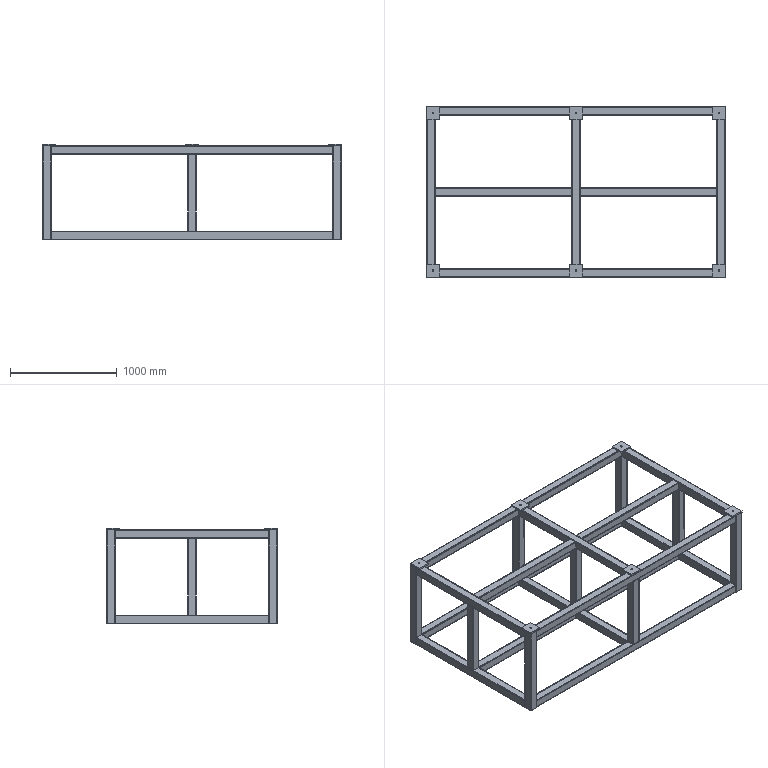Part | STEP file | Part3_default<as machined> | 29 solids | 466 faces | box 2800 x 1600 x 895 mm | volume 31350509 mm3 | plane 266 | cylinder 200 | commonest cylinder face diameters 6.4 x92 12.8 x92 17.5 x16